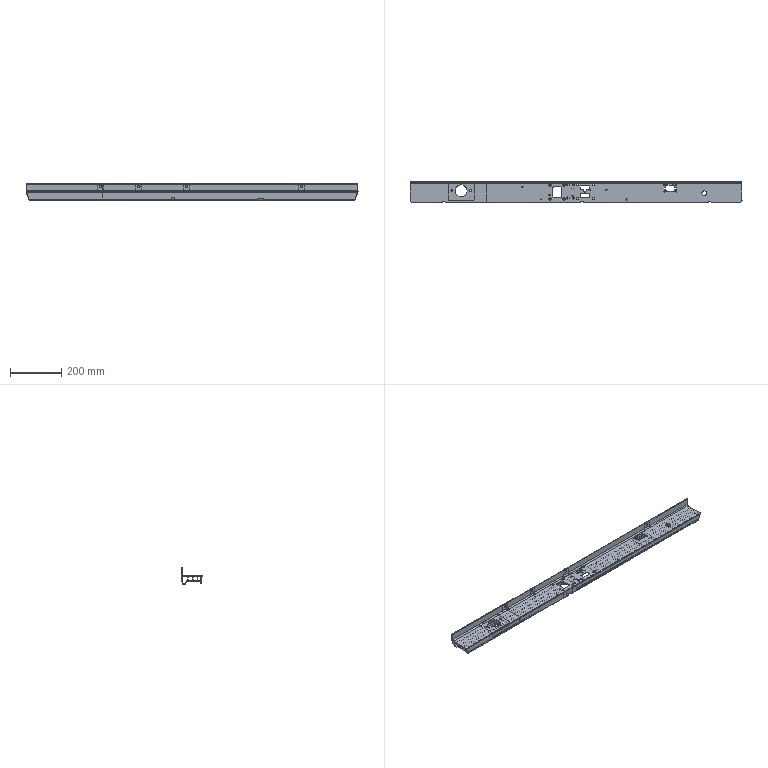NC program | NX | posted with a generic post | part box 1301 x 81.1 x 63 mm
Lines 1 to 1193 of 19815:
N10 G17 G21 G94 G90
(FLOOR_WALL_COPY_COPY , TOOL : D10)
N12 T10 M6
N14 G54
N16 G17 G0 G90 X127.709 Y30.2 B0. C0. S6000 M3
N18 G43 Z30. H10
N20 Z1.5
N22 G94 G1 X107.257 Z0.428 F1000.
N24 Y28.734 Z0.351
N26 X132.857 Z-0.991
N28 X158.457 F2500.
N30 Y30.2
N32 X107.257
N34 Y28.734
N36 X132.857
N38 Y24.234
N40 X162.957
N42 Y34.7
N44 X102.757
N46 Y24.234
N48 X132.857
N50 G2 X133.724 Y23.734 R1.
N52 G1 X134.301 Y22.734
N54 Z0.509
N56 G0 X161.859
N58 G1 Z-0.991 F1000.
N60 X162.957 Y23.368
N62 G3 X163.457 Y24.234 R1.
N64 G1 Y35.2 F2500.
N66 X102.257
N68 Y24.234
N70 G3 X102.757 Y23.368 R1.
N72 G1 X103.856 Y22.734
N74 Z0.509
N76 G0 X127.144 Y30.2
N78 G1 X107.257 Z-0.533 F1000.
N80 Y28.168 Z-0.639
N82 X132.857 Z-1.981
N84 X158.457 F2500.
N86 Y30.2
N88 X107.257
N90 Y28.168
N92 X132.857
N94 Y23.668
N96 X162.957
N98 Y34.7
N100 X102.757
N102 Y23.668
N104 X132.857
N106 G2 X133.724 Y23.168 R1.
N108 G1 X134.301 Y22.168
N110 Z-0.481
N112 G0 X161.859
N114 G1 Z-1.981 F1000.
N116 X162.957 Y22.802
N118 G3 X163.457 Y23.668 R1.
N120 G1 Y35.2 F2500.
N122 X102.257
N124 Y23.668
N126 G3 X102.757 Y22.802 R1.
N128 G1 X103.856 Y22.168
N130 Z-0.481
N132 G0 X126.578 Y30.2
N134 G1 X107.257 Z-1.493 F1000.
N136 Y27.602 Z-1.63
N138 X132.857 Z-2.971
N140 X158.457 F2500.
N142 Y30.2
N144 X107.257
N146 Y27.602
N148 X132.857
N150 Y23.102
N152 X162.957
N154 Y34.7
N156 X102.757
N158 Y23.102
N160 X132.857
N162 G2 X133.724 Y22.602 R1.
N164 G1 X134.301 Y21.602
N166 Z-1.471
N168 G0 X161.859
N170 G1 Z-2.971 F1000.
N172 X162.957 Y22.236
N174 G3 X163.457 Y23.102 R1.
N176 G1 Y35.2 F2500.
N178 X102.257
N180 Y23.102
N182 G3 X102.757 Y22.236 R1.
N184 G1 X103.856 Y21.602
N186 Z-1.471
N188 G0 X126.012 Y30.2
N190 G1 X107.257 Z-2.454 F1000.
N192 Y27.036 Z-2.62
N194 X132.857 Z-3.962
N196 X158.457 F2500.
N198 Y30.2
N200 X107.257
N202 Y27.036
N204 X132.857
N206 Y22.536
N208 X162.957
N210 Y34.7
N212 X102.757
N214 Y22.536
N216 X132.857
N218 G2 X133.724 Y22.036 R1.
N220 G1 X134.301 Y21.036
N222 Z-2.462
N224 G0 X161.859
N226 G1 Z-3.962 F1000.
N228 X162.957 Y21.67
N230 G3 X163.457 Y22.536 R1.
N232 G1 Y35.2 F2500.
N234 X102.257
N236 Y22.536
N238 G3 X102.757 Y21.67 R1.
N240 G1 X103.856 Y21.036
N242 Z-2.462
N244 G0 X140.409 Y26.47
N246 G1 X158.457 Z-3.407 F1000.
N248 Y30.34 Z-3.61
N250 X132.857 Z-4.952
N252 X107.257 F2500.
N254 Y26.47
N256 X158.457
N258 Y30.34
N260 X132.857
N262 Y34.84
N264 X102.757
N266 Y21.97
N268 X162.957
N270 Y34.84
N272 X132.857
N274 Z-3.452
N276 G0 X104.257 Y33.34
N278 G1 Z-4.952 F1000.
N280 X102.324 Y35.09
N282 G3 X102.257 Y34.84 R0.5
N284 G1 Y21.97 F2500.
N286 G3 X102.757 Y21.104 R1.
N288 G1 X103.856 Y20.47
N290 Z-3.452
N292 G0 X161.859
N294 G1 Z-4.952 F1000.
N296 X162.957 Y21.104
N298 G3 X163.457 Y21.97 R1.
N300 G1 Y34.84 F2500.
N302 G3 X163.391 Y35.09 R0.5
N304 G1 X161.457 Y33.34
N306 Z-3.452
N308 G0 X140.409 Y25.904
N310 G1 X158.457 Z-4.398 F1000.
N312 Y29.774 Z-4.601
N314 X132.857 Z-5.942
N316 X107.257 F2500.
N318 Y25.904
N320 X158.457
N322 Y29.774
N324 X132.857
N326 Y34.274
N328 X102.757
N330 Y21.404
N332 X162.957
N334 Y34.274
N336 X132.857
N338 G2 X132.424 Y34.524 R0.5
N340 G1 Z-4.442
N342 G0 X104.257 Y32.774
N344 G1 Z-5.942 F1000.
N346 X102.757 Y35.14
N348 G3 X102.257 Y34.274 R1.
N350 G1 Y21.404 F2500.
N352 G3 X102.757 Y20.538 R1.
N354 G1 X103.856 Y19.904
N356 Z-4.442
N358 G0 X161.859
N360 G1 Z-5.942 F1000.
N362 X162.957 Y20.538
N364 G3 X163.457 Y21.404 R1.
N366 G1 Y34.274 F2500.
N368 G3 X162.957 Y35.14 R1.
N370 G1 X161.457 Y32.774
N372 Z-4.442
N374 G0 X140.409 Y25.339
N376 G1 X158.457 Z-5.388 F1000.
N378 Y29.208 Z-5.591
N380 X132.857 Z-6.932
N382 X107.257 F2500.
N384 Y25.339
N386 X158.457
N388 Y29.208
N390 X132.857
N392 Y33.708
N394 X102.757
N396 Y20.839
N398 X162.957
N400 Y33.708
N402 X132.857
N404 G2 X131.991 Y34.208 R1.
N406 G1 Z-5.432
N408 G0 X104.257 Y32.208
N410 G1 Z-6.932 F1000.
N412 X102.757 Y34.574
N414 G3 X102.257 Y33.708 R1.
N416 G1 Y20.839 F2500.
N418 G3 X102.757 Y19.973 R1.
N420 G1 X103.856 Y19.339
N422 Z-5.432
N424 G0 X161.859
N426 G1 Z-6.932 F1000.
N428 X162.957 Y19.973
N430 G3 X163.457 Y20.839 R1.
N432 G1 Y33.708 F2500.
N434 G3 X162.957 Y34.574 R1.
N436 G1 X161.457 Y32.208
N438 Z-5.432
N440 G0 X140.409 Y24.773
N442 G1 X158.457 Z-6.378 F1000.
N444 Y28.642 Z-6.581
N446 X132.857 Z-7.923
N448 X107.257 F2500.
N450 Y24.773
N452 X158.457
N454 Y28.642
N456 X132.857
N458 Y33.142
N460 X102.757
N462 Y20.273
N464 X162.957
N466 Y33.142
N468 X132.857
N470 G2 X131.991 Y33.642 R1.
N472 G1 Z-6.423
N474 G0 X104.257 Y31.642
N476 G1 Z-7.923 F1000.
N478 X102.757 Y34.008
N480 G3 X102.257 Y33.142 R1.
N482 G1 Y20.273 F2500.
N484 G3 X102.757 Y19.407 R1.
N486 G1 X103.856 Y18.773
N488 Z-6.423
N490 G0 X161.859
N492 G1 Z-7.923 F1000.
N494 X162.957 Y19.407
N496 G3 X163.457 Y20.273 R1.
N498 G1 Y33.142 F2500.
N500 G3 X162.957 Y34.008 R1.
N502 G1 X161.457 Y31.642
N504 Z-6.423
N506 G0 X140.409 Y24.207
N508 G1 X158.457 Z-7.369 F1000.
N510 Y28.076 Z-7.571
N512 X132.857 Z-8.913
N514 X107.257 F2500.
N516 Y24.207
N518 X158.457
N520 Y28.076
N522 X132.857
N524 Y32.576
N526 X102.757
N528 Y19.707
N530 X162.957
N532 Y32.576
N534 X132.857
N536 G2 X131.991 Y33.076 R1.
N538 G1 Z-7.413
N540 G0 X104.257 Y31.076
N542 G1 Z-8.913 F1000.
N544 X102.757 Y33.442
N546 G3 X102.257 Y32.576 R1.
N548 G1 Y19.707 F2500.
N550 G3 X102.757 Y18.841 R1.
N552 G1 X103.856 Y18.207
N554 Z-7.413
N556 G0 X161.859
N558 G1 Z-8.913 F1000.
N560 X162.957 Y18.841
N562 G3 X163.457 Y19.707 R1.
N564 G1 Y32.576 F2500.
N566 G3 X162.957 Y33.442 R1.
N568 G1 X161.457 Y31.076
N570 Z-7.413
N572 G0 X141.011 Y23.039
N574 G1 X158.457 Z-8.327 F1000.
N576 Y27.51 Z-8.562
N578 X132.857 Z-9.903
N580 X107.257 F2500.
N582 Y23.039
N584 X158.457
N586 Y27.51
N588 X132.857
N590 Y32.01
N592 X102.757
N594 Y18.539
N596 X162.957
N598 Y32.01
N600 X132.857
N602 G2 X131.991 Y32.51 R1.
N604 G1 X131.414 Y33.51
N606 Z-8.403
N608 G0 X103.856
N610 G1 Z-9.903 F1000.
N612 X102.757 Y32.876
N614 G3 X102.257 Y32.01 R1.
N616 G1 Y18.539 F2500.
N618 G3 X102.757 Y17.673 R1.
N620 G1 X103.856 Y17.039
N622 Z-8.403
N624 G0 X161.859
N626 G1 Z-9.903 F1000.
N628 X162.957 Y17.673
N630 G3 X163.457 Y18.539 R1.
N632 G1 Y32.01 F2500.
N634 G3 X162.957 Y32.876 R1.
N636 G1 X161.859 Y33.51
N638 Z-8.403
N640 G0 X125.584 Y9.4
N642 G1 X148.957 Z-9.628 F1000.
N644 Y17.444 Z-10.05
N646 X132.857 Z-10.894
N648 X116.757 F2500.
N650 Y9.4
N652 X148.957
N654 Y17.444
N656 X132.857
N658 Y24.444
N660 X109.757
N662 Y2.4
N664 X155.957
N666 Y24.444
N668 X132.857
N670 Y31.444
N672 X102.757
N674 Y-4.6
N676 X162.957
N678 Y31.444
N680 X132.857
N682 G2 X131.991 Y31.944 R1.
N684 G1 X131.414 Y32.944
N686 Z-9.394
N688 G0 X103.856
N690 G1 Z-10.894 F1000.
N692 X102.757 Y32.31
N694 G3 X102.257 Y31.444 R1.
N696 G1 Y-5.1 F2500.
N698 X163.457
N700 Y31.444
N702 G3 X162.957 Y32.31 R1.
N704 G1 X161.859 Y32.944
N706 Z-9.394
N708 G0 X125.018 Y9.4
N710 G1 X148.957 Z-10.648 F1000.
N712 Y16.878 Z-11.04
N714 X132.857 Z-11.884
N716 X116.757 F2500.
N718 Y9.4
N720 X148.957
N722 Y16.878
N724 X132.857
N726 Y23.878
N728 X109.757
N730 Y2.4
N732 X155.957
N734 Y23.878
N736 X132.857
N738 Y30.878
N740 X102.757
N742 Y-4.6
N744 X162.957
N746 Y30.878
N748 X132.857
N750 G2 X131.991 Y31.378 R1.
N752 G1 X131.414 Y32.378
N754 Z-10.384
N756 G0 X103.856
N758 G1 Z-11.884 F1000.
N760 X102.757 Y31.745
N762 G3 X102.257 Y30.878 R1.
N764 G1 Y-5.1 F2500.
N766 X163.457
N768 Y30.878
N770 G3 X162.957 Y31.745 R1.
N772 G1 X161.859 Y32.378
N774 Z-10.384
N776 G0 X124.452 Y9.4
N778 G1 X148.957 Z-11.668 F1000.
N780 Y16.313 Z-12.031
N782 X132.857 Z-12.874
N784 X116.757 F2500.
N786 Y9.4
N788 X148.957
N790 Y16.313
N792 X132.857
N794 Y23.313
N796 X109.757
N798 Y2.4
N800 X155.957
N802 Y23.313
N804 X132.857
N806 Y30.313
N808 X102.757
N810 Y-4.6
N812 X162.957
N814 Y30.313
N816 X132.857
N818 G2 X131.991 Y30.813 R1.
N820 G1 X131.414 Y31.813
N822 Z-11.374
N824 G0 X103.856
N826 G1 Z-12.874 F1000.
N828 X102.757 Y31.179
N830 G3 X102.257 Y30.313 R1.
N832 G1 Y-5.1 F2500.
N834 X163.457
N836 Y30.313
N838 G3 X162.957 Y31.179 R1.
N840 G1 X161.859 Y31.813
N842 Z-11.374
N844 G0 X125.482 Y3.647
N846 G1 X107.257 Z-12.329 F1000.
N848 Y-0.047 Z-12.523
N850 X132.857 Z-13.865
N852 X158.457 F2500.
N854 Y3.647
N856 X107.257
N858 Y-0.047
N860 X132.857
N862 Y-4.547
N864 X162.957
N866 Y8.147
N868 X102.757
N870 Y-4.547
N872 X132.857
N874 G2 X133.107 Y-4.614 R0.5
N876 G1 Z-12.365
N878 G0 X161.457 Y-3.047
N880 G1 Z-13.865 F1000.
N882 X163.207 Y-4.98
N884 G3 X163.457 Y-4.547 R0.5
N886 G1 Y8.147 F2500.
N888 G3 X162.957 Y9.013 R1.
N890 G1 X161.859 Y9.647
N892 Z-12.365
N894 G0 X103.856
N896 G1 Z-13.865 F1000.
N898 X102.757 Y9.013
N900 G3 X102.257 Y8.147 R1.
N902 G1 Y-4.547 F2500.
N904 G3 X102.507 Y-4.98 R0.5
N906 G1 X104.257 Y-3.047
N908 Z-12.365
N910 G0 X126.166 Y3.305
N912 G1 X107.257 Z-13.356 F1000.
N914 Y0.295 Z-13.513
N916 X132.857 Z-14.855
N918 X158.457 F2500.
N920 Y3.305
N922 X107.257
N924 Y0.295
N926 X132.857
N928 Y-4.205
N930 X162.957
N932 Y7.805
N934 X102.757
N936 Y-4.205
N938 X132.857
N940 G2 X133.291 Y-4.455 R0.5
N942 G1 Z-13.355
N944 G0 X161.457 Y-2.705
N946 G1 Z-14.855 F1000.
N948 X162.957 Y-5.071
N950 G3 X163.457 Y-4.205 R1.
N952 G1 Y7.805 F2500.
N954 G3 X162.957 Y8.671 R1.
N956 G1 X161.859 Y9.305
N958 Z-13.355
N960 G0 X103.856
N962 G1 Z-14.855 F1000.
N964 X102.757 Y8.671
N966 G3 X102.257 Y7.805 R1.
N968 G1 Y-4.205 F2500.
N970 G3 X102.757 Y-5.071 R1.
N972 G1 X104.257 Y-2.705
N974 Z-13.355
N976 G0 X126.175 Y3.3
N978 G1 X107.257 Z-14.346 F1000.
N980 Y0.3 Z-14.504
N982 X132.857 Z-15.845
N984 X158.457 F2500.
N986 Y3.3
N988 X107.257
N990 Y0.3
N992 X132.857
N994 Y-4.2
N996 X162.957
N998 Y7.8
N1000 X102.757
N1002 Y-4.2
N1004 X132.857
N1006 G2 X133.291 Y-4.45 R0.5
N1008 G1 Z-14.345
N1010 G0 X161.457 Y-2.7
N1012 G1 Z-15.845 F1000.
N1014 X162.957 Y-5.066
N1016 G3 X163.457 Y-4.2 R1.
N1018 G1 Y7.8 F2500.
N1020 G3 X162.957 Y8.666 R1.
N1022 G1 X161.859 Y9.3
N1024 Z-14.345
N1026 G0 X103.856
N1028 G1 Z-15.845 F1000.
N1030 X102.757 Y8.666
N1032 G3 X102.257 Y7.8 R1.
N1034 G1 Y-4.2 F2500.
N1036 G3 X102.757 Y-5.066 R1.
N1038 G1 X104.257 Y-2.7
N1040 Z-14.345
N1042 G0 X126.175 Y3.3
N1044 G1 X107.257 Z-15.337 F1000.
N1046 Y0.3 Z-15.494
N1048 X132.857 Z-16.836
N1050 X158.457 F2500.
N1052 Y3.3
N1054 X107.257
N1056 Y0.3
N1058 X132.857
N1060 Y-4.2
N1062 X162.957
N1064 Y7.8
N1066 X102.757
N1068 Y-4.2
N1070 X132.857
N1072 G2 X133.291 Y-4.45 R0.5
N1074 G1 Z-15.336
N1076 G0 X161.457 Y-2.7
N1078 G1 Z-16.836 F1000.
N1080 X162.957 Y-5.066
N1082 G3 X163.457 Y-4.2 R1.
N1084 G1 Y7.8 F2500.
N1086 G3 X162.957 Y8.666 R1.
N1088 G1 X161.859 Y9.3
N1090 Z-15.336
N1092 G0 X103.856
N1094 G1 Z-16.836 F1000.
N1096 X102.757 Y8.666
N1098 G3 X102.257 Y7.8 R1.
N1100 G1 Y-4.2 F2500.
N1102 G3 X102.757 Y-5.066 R1.
N1104 G1 X104.257 Y-2.7
N1106 Z-15.336
N1108 G0 X126.175 Y3.3
N1110 G1 X107.257 Z-16.327 F1000.
N1112 Y0.3 Z-16.484
N1114 X132.857 Z-17.826
N1116 X158.457 F2500.
N1118 Y3.3
N1120 X107.257
N1122 Y0.3
N1124 X132.857
N1126 Y-4.2
N1128 X162.957
N1130 Y7.8
N1132 X102.757
N1134 Y-4.2
N1136 X132.857
N1138 G2 X133.291 Y-4.45 R0.5
N1140 G1 Z-16.326
N1142 G0 X161.457 Y-2.7
N1144 G1 Z-17.826 F1000.
N1146 X162.957 Y-5.066
N1148 G3 X163.457 Y-4.2 R1.
N1150 G1 Y7.8 F2500.
N1152 G3 X162.957 Y8.666 R1.
N1154 G1 X161.859 Y9.3
N1156 Z-16.326
N1158 G0 X103.856
N1160 G1 Z-17.826 F1000.
N1162 X102.757 Y8.666
N1164 G3 X102.257 Y7.8 R1.
N1166 G1 Y-4.2 F2500.
N1168 G3 X102.757 Y-5.066 R1.
N1170 G1 X104.257 Y-2.7
N1172 Z-16.326
N1174 G0 X126.175 Y3.3
N1176 G1 X107.257 Z-17.317 F1000.
N1178 Y0.3 Z-17.475
N1180 X132.857 Z-18.816
N1182 X158.457 F2500.
N1184 Y3.3
N1186 X107.257
N1188 Y0.3
N1190 X132.857
N1192 Y-4.2
N1194 X162.957
N1196 Y7.8
N1198 X102.757
N1200 Y-4.2
N1202 X132.857
N1204 G2 X133.291 Y-4.45 R0.5
N1206 G1 Z-17.316
N1208 G0 X161.457 Y-2.7
N1210 G1 Z-18.816 F1000.
N1212 X162.957 Y-5.066
N1214 G3 X163.457 Y-4.2 R1.
N1216 G1 Y7.8 F2500.
N1218 G3 X162.957 Y8.666 R1.
N1220 G1 X161.859 Y9.3
N1222 Z-17.316
N1224 G0 X103.856
N1226 G1 Z-18.816 F1000.
N1228 X102.757 Y8.666
N1230 G3 X102.257 Y7.8 R1.
N1232 G1 Y-4.2 F2500.
N1234 G3 X102.757 Y-5.066 R1.
N1236 G1 X104.257 Y-2.7
N1238 Z-17.316
N1240 G0 X126.175 Y3.3
N1242 G1 X107.257 Z-18.308 F1000.
N1244 Y0.3 Z-18.465
N1246 X132.857 Z-19.807
N1248 X158.457 F2500.
N1250 Y3.3
N1252 X107.257
N1254 Y0.3
N1256 X132.857
N1258 Y-4.2
N1260 X162.957
N1262 Y7.8
N1264 X102.757
N1266 Y-4.2
N1268 X132.857
N1270 G2 X133.291 Y-4.45 R0.5
N1272 G1 Z-18.307
N1274 G0 X161.457 Y-2.7
N1276 G1 Z-19.807 F1000.
N1278 X162.957 Y-5.066
N1280 G3 X163.457 Y-4.2 R1.
N1282 G1 Y7.8 F2500.
N1284 G3 X162.957 Y8.666 R1.
N1286 G1 X161.859 Y9.3
N1288 Z-18.307
N1290 G0 X103.856
N1292 G1 Z-19.807 F1000.
N1294 X102.757 Y8.666
N1296 G3 X102.257 Y7.8 R1.
N1298 G1 Y-4.2 F2500.
N1300 G3 X102.757 Y-5.066 R1.
N1302 G1 X104.257 Y-2.7
N1304 Z-18.307
N1306 G0 X126.175 Y3.3
N1308 G1 X107.257 Z-19.298 F1000.
N1310 Y0.3 Z-19.455
N1312 X132.857 Z-20.797
N1314 X158.457 F2500.
N1316 Y3.3
N1318 X107.257
N1320 Y0.3
N1322 X132.857
N1324 Y-4.2
N1326 X162.957
N1328 Y7.8
N1330 X102.757
N1332 Y-4.2
N1334 X132.857
N1336 G2 X133.291 Y-4.45 R0.5
N1338 G1 Z-19.297
N1340 G0 X161.457 Y-2.7
N1342 G1 Z-20.797 F1000.
N1344 X162.957 Y-5.066
N1346 G3 X163.457 Y-4.2 R1.
N1348 G1 Y7.8 F2500.
N1350 G3 X162.957 Y8.666 R1.
N1352 G1 X161.859 Y9.3
N1354 Z-19.297
N1356 G0 X103.856
N1358 G1 Z-20.797 F1000.
N1360 X102.757 Y8.666
N1362 G3 X102.257 Y7.8 R1.
N1364 G1 Y-4.2 F2500.
N1366 G3 X102.757 Y-5.066 R1.
N1368 G1 X104.257 Y-2.7
N1370 Z-19.297
N1372 G0 X126.175 Y3.3
N1374 G1 X107.257 Z-20.288 F1000.
N1376 Y0.3 Z-20.446
N1378 X132.857 Z-21.787
N1380 X158.457 F2500.
N1382 Y3.3
N1384 X107.257
N1386 Y0.3
N1388 X132.857
N1390 Y-4.2
N1392 X162.957
N1394 Y7.8
N1396 X102.757
N1398 Y-4.2
N1400 X132.857
N1402 G2 X133.291 Y-4.45 R0.5
N1404 G1 Z-20.287
N1406 G0 X161.457 Y-2.7
N1408 G1 Z-21.787 F1000.
N1410 X162.957 Y-5.066
N1412 G3 X163.457 Y-4.2 R1.
N1414 G1 Y7.8 F2500.
N1416 G3 X162.957 Y8.666 R1.
N1418 G1 X161.859 Y9.3
N1420 Z-20.287
N1422 G0 X103.856
N1424 G1 Z-21.787 F1000.
N1426 X102.757 Y8.666
N1428 G3 X102.257 Y7.8 R1.
N1430 G1 Y-4.2 F2500.
N1432 G3 X102.757 Y-5.066 R1.
N1434 G1 X104.257 Y-2.7
N1436 Z-20.287
N1438 G0 X126.175 Y3.3
N1440 G1 X107.257 Z-21.279 F1000.
N1442 Y0.3 Z-21.436
N1444 X132.857 Z-22.777
N1446 X158.457 F2500.
N1448 Y3.3
N1450 X107.257
N1452 Y0.3
N1454 X132.857
N1456 Y-4.2
N1458 X162.957
N1460 Y7.8
N1462 X102.757
N1464 Y-4.2
N1466 X132.857
N1468 G2 X133.291 Y-4.45 R0.5
N1470 G1 Z-21.277
N1472 G0 X161.457 Y-2.7
N1474 G1 Z-22.777 F1000.
N1476 X162.957 Y-5.066
N1478 G3 X163.457 Y-4.2 R1.
N1480 G1 Y7.8 F2500.
N1482 G3 X162.957 Y8.666 R1.
N1484 G1 X161.859 Y9.3
N1486 Z-21.277
N1488 G0 X103.856
N1490 G1 Z-22.777 F1000.
N1492 X102.757 Y8.666
N1494 G3 X102.257 Y7.8 R1.
N1496 G1 Y-4.2 F2500.
N1498 G3 X102.757 Y-5.066 R1.
N1500 G1 X104.257 Y-2.7
N1502 Z-21.277
N1504 G0 X126.175 Y3.3
N1506 G1 X107.257 Z-22.269 F1000.
N1508 Y0.3 Z-22.426
N1510 X132.857 Z-23.768
N1512 X158.457 F2500.
N1514 Y3.3
N1516 X107.257
N1518 Y0.3
N1520 X132.857
N1522 Y-4.2
N1524 X162.957
N1526 Y7.8
N1528 X102.757
N1530 Y-4.2
N1532 X132.857
N1534 G2 X133.291 Y-4.45 R0.5
N1536 G1 Z-22.268
N1538 G0 X161.457 Y-2.7
N1540 G1 Z-23.768 F1000.
N1542 X162.957 Y-5.066
N1544 G3 X163.457 Y-4.2 R1.
N1546 G1 Y7.8 F2500.
N1548 G3 X162.957 Y8.666 R1.
N1550 G1 X161.859 Y9.3
N1552 Z-22.268
N1554 G0 X103.856
N1556 G1 Z-23.768 F1000.
N1558 X102.757 Y8.666
N1560 G3 X102.257 Y7.8 R1.
N1562 G1 Y-4.2 F2500.
N1564 G3 X102.757 Y-5.066 R1.
N1566 G1 X104.257 Y-2.7
N1568 Z-22.268
N1570 G0 X126.175 Y3.3
N1572 G1 X107.257 Z-23.259 F1000.
N1574 Y0.3 Z-23.416
N1576 X132.857 Z-24.758
N1578 X158.457 F2500.
N1580 Y3.3
N1582 X107.257
N1584 Y0.3
N1586 X132.857
N1588 Y-4.2
N1590 X162.957
N1592 Y7.8
N1594 X102.757
N1596 Y-4.2
N1598 X132.857
N1600 G2 X133.291 Y-4.45 R0.5
N1602 G1 Z-23.258
N1604 G0 X161.457 Y-2.7
N1606 G1 Z-24.758 F1000.
N1608 X162.957 Y-5.066
N1610 G3 X163.457 Y-4.2 R1.
N1612 G1 Y7.8 F2500.
N1614 G3 X162.957 Y8.666 R1.
N1616 G1 X161.859 Y9.3
N1618 Z-23.258
N1620 G0 X103.856
N1622 G1 Z-24.758 F1000.
N1624 X102.757 Y8.666
N1626 G3 X102.257 Y7.8 R1.
N1628 G1 Y-4.2 F2500.
N1630 G3 X102.757 Y-5.066 R1.
N1632 G1 X104.257 Y-2.7
N1634 Z-23.258
N1636 G0 X126.175 Y3.3
N1638 G1 X107.257 Z-24.25 F1000.
N1640 Y0.3 Z-24.407
N1642 X132.857 Z-25.748
N1644 X158.457 F2500.
N1646 Y3.3
N1648 X107.257
N1650 Y0.3
N1652 X132.857
N1654 Y-4.2
N1656 X162.957
N1658 Y7.8
N1660 X102.757
N1662 Y-4.2
N1664 X132.857
N1666 G2 X133.291 Y-4.45 R0.5
N1668 G1 Z-24.248
N1670 G0 X161.457 Y-2.7
N1672 G1 Z-25.748 F1000.
N1674 X162.957 Y-5.066
N1676 G3 X163.457 Y-4.2 R1.
N1678 G1 Y7.8 F2500.
N1680 G3 X162.957 Y8.666 R1.
N1682 G1 X161.859 Y9.3
N1684 Z-24.248
N1686 G0 X103.856
N1688 G1 Z-25.748 F1000.
N1690 X102.757 Y8.666
N1692 G3 X102.257 Y7.8 R1.
N1694 G1 Y-4.2 F2500.
N1696 G3 X102.757 Y-5.066 R1.
N1698 G1 X104.257 Y-2.7
N1700 Z-24.248
N1702 G0 X126.175 Y3.3
N1704 G1 X107.257 Z-25.24 F1000.
N1706 Y0.3 Z-25.397
N1708 X132.857 Z-26.739
N1710 X158.457 F2500.
N1712 Y3.3
N1714 X107.257
N1716 Y0.3
N1718 X132.857
N1720 Y-4.2
N1722 X162.957
N1724 Y7.8
N1726 X102.757
N1728 Y-4.2
N1730 X132.857
N1732 G2 X133.291 Y-4.45 R0.5
N1734 G1 Z-25.239
N1736 G0 X161.457 Y-2.7
N1738 G1 Z-26.739 F1000.
N1740 X162.957 Y-5.066
N1742 G3 X163.457 Y-4.2 R1.
N1744 G1 Y7.8 F2500.
N1746 G3 X162.957 Y8.666 R1.
N1748 G1 X161.859 Y9.3
N1750 Z-25.239
N1752 G0 X103.856
N1754 G1 Z-26.739 F1000.
N1756 X102.757 Y8.666
N1758 G3 X102.257 Y7.8 R1.
N1760 G1 Y-4.2 F2500.
N1762 G3 X102.757 Y-5.066 R1.
N1764 G1 X104.257 Y-2.7
N1766 Z-25.239
N1768 G0 X126.175 Y3.3
N1770 G1 X107.257 Z-26.23 F1000.
N1772 Y0.3 Z-26.387
N1774 X132.857 Z-27.729
N1776 X158.457 F2500.
N1778 Y3.3
N1780 X107.257
N1782 Y0.3
N1784 X132.857
N1786 Y-4.2
N1788 X162.957
N1790 Y7.8
N1792 X102.757
N1794 Y-4.2
N1796 X132.857
N1798 G2 X133.291 Y-4.45 R0.5
N1800 G1 Z-26.229
N1802 G0 X161.457 Y-2.7
N1804 G1 Z-27.729 F1000.
N1806 X162.957 Y-5.066
N1808 G3 X163.457 Y-4.2 R1.
N1810 G1 Y7.8 F2500.
N1812 G3 X162.957 Y8.666 R1.
N1814 G1 X161.859 Y9.3
N1816 Z-26.229
N1818 G0 X103.856
N1820 G1 Z-27.729 F1000.
N1822 X102.757 Y8.666
N1824 G3 X102.257 Y7.8 R1.
N1826 G1 Y-4.2 F2500.
N1828 G3 X102.757 Y-5.066 R1.
N1830 G1 X104.257 Y-2.7
N1832 Z-26.229
N1834 G0 X126.163 Y3.3
N1836 G1 X107.257 Z-27.22 F1000.
N1838 Y0.288 Z-27.378
N1840 X132.857 Z-28.719
N1842 X158.457 F2500.
N1844 Y3.3
N1846 X107.257
N1848 Y0.288
N1850 X132.857
N1852 Y-4.212
N1854 X162.957
N1856 Y7.8
N1858 X102.757
N1860 Y-4.212
N1862 X132.857
N1864 G2 X133.291 Y-4.462 R0.5
N1866 G1 Z-27.219
N1868 G0 X161.457 Y-2.712
N1870 G1 Z-28.719 F1000.
N1872 X162.957 Y-5.078
N1874 G3 X163.457 Y-4.212 R1.
N1876 G1 Y7.8 F2500.
N1878 G3 X162.957 Y8.666 R1.
N1880 G1 X161.859 Y9.3
N1882 Z-27.219
N1884 G0 X103.856
N1886 G1 Z-28.719 F1000.
N1888 X102.757 Y8.666
N1890 G3 X102.257 Y7.8 R1.
N1892 G1 Y-4.212 F2500.
N1894 G3 X102.757 Y-5.078 R1.
N1896 G1 X104.257 Y-2.712
N1898 Z-27.219
N1900 G0 X125.746 Y3.322
N1902 G1 X107.257 Z-28.188 F1000.
N1904 Y-0.107 Z-28.368
N1906 X132.857 Z-29.71
N1908 X158.457 F2500.
N1910 Y3.322
N1912 X107.257
N1914 Y-0.107
N1916 X132.857
N1918 Y-4.607
N1920 X162.957
N1922 Y7.822
N1924 X102.757
N1926 Y-4.607
N1928 X132.857
N1930 Z-28.21
N1932 G0 X161.457 Y-3.107
N1934 G1 Z-29.71 F1000.
N1936 X163.207 Y-5.04
N1938 G3 X163.457 Y-4.607 R0.5
N1940 G1 Y7.822 F2500.
N1942 G3 X162.957 Y8.688 R1.
N1944 G1 X161.859 Y9.322
N1946 Z-28.21
N1948 G0 X103.856
N1950 G1 Z-29.71 F1000.
N1952 X102.757 Y8.688
N1954 G3 X102.257 Y7.822 R1.
N1956 G1 Y-4.607 F2500.
N1958 G3 X102.507 Y-5.04 R0.5
N1960 G1 X104.257 Y-3.107
N1962 Z-28.21
N1964 G0 Z30.
N1966 X133.333 Y20.953
N1968 Z-11.374
N1970 G1 X155.957 Z-12.56 F1000.
N1972 Y22.747 Z-12.654
N1974 X132.857 Z-13.865
N1976 X109.757 F2500.
N1978 Y20.953
N1980 X155.957
N1982 Y22.747
N1984 X132.857
N1986 Y29.747
N1988 X102.757
N1990 Y13.953
N1992 X162.957
N1994 Y29.747
N1996 X132.857
N1998 G2 X131.991 Y30.247 R1.
N2000 G1 X131.414 Y31.247
N2002 Z-12.365
N2004 G0 X103.856
N2006 G1 Z-13.865 F1000.
N2008 X102.757 Y30.613
N2010 G3 X102.257 Y29.747 R1.
N2012 G1 Y13.953 F2500.
N2014 G3 X102.757 Y13.087 R1.
N2016 G1 X103.856 Y12.453
N2018 Z-12.365
N2020 G0 X161.859
N2022 G1 Z-13.865 F1000.
N2024 X162.957 Y13.087
N2026 G3 X163.457 Y13.953 R1.
N2028 G1 Y29.747 F2500.
N2030 G3 X162.957 Y30.613 R1.
N2032 G1 X161.859 Y31.247
N2034 Z-12.365
N2036 G0 X132.425 Y21.295
N2038 G1 X155.957 Z-13.598 F1000.
N2040 Y22.181 Z-13.644
N2042 X132.857 Z-14.855
N2044 X109.757 F2500.
N2046 Y21.295
N2048 X155.957
N2050 Y22.181
N2052 X132.857
N2054 Y29.181
N2056 X102.757
N2058 Y14.295
N2060 X162.957
N2062 Y29.181
N2064 X132.857
N2066 G2 X131.991 Y29.681 R1.
N2068 G1 X131.414 Y30.681
N2070 Z-13.355
N2072 G0 X103.856
N2074 G1 Z-14.855 F1000.
N2076 X102.757 Y30.047
N2078 G3 X102.257 Y29.181 R1.
N2080 G1 Y14.295 F2500.
N2082 G3 X102.757 Y13.429 R1.
N2084 G1 X103.856 Y12.795
N2086 Z-13.355
N2088 G0 X161.859
N2090 G1 Z-14.855 F1000.
N2092 X162.957 Y13.429
N2094 G3 X163.457 Y14.295 R1.
N2096 G1 Y29.181 F2500.
N2098 G3 X162.957 Y30.047 R1.
N2100 G1 X161.859 Y30.681
N2102 Z-13.355
N2104 G0 X133.861 Y21.615
N2106 G1 X109.757 Z-14.618 F1000.
N2108 Y21.3 Z-14.635
N2110 X132.857 Z-15.845
N2112 X155.957 F2500.
N2114 Y21.615
N2116 X109.757
N2118 Y21.3
N2120 X132.857
N2122 Y14.3
N2124 X162.957
N2126 Y28.615
N2128 X102.757
N2130 Y14.3
N2132 X132.857
N2134 G2 X133.724 Y13.8 R1.
N2136 G1 X134.301 Y12.8
N2138 Z-14.345
N2140 G0 X161.859
N2142 G1 Z-15.845 F1000.
N2144 X162.957 Y13.434
N2146 G3 X163.457 Y14.3 R1.
N2148 G1 Y28.615 F2500.
N2150 G3 X162.957 Y29.481 R1.
N2152 G1 X161.859 Y30.115
N2154 Z-14.345
N2156 G0 X103.856
N2158 G1 Z-15.845 F1000.
N2160 X102.757 Y29.481
N2162 G3 X102.257 Y28.615 R1.
N2164 G1 Y14.3 F2500.
N2166 G3 X102.757 Y13.434 R1.
N2168 G1 X103.856 Y12.8
N2170 Z-14.345
N2172 G0 X141.288 Y18.8
N2174 G1 X158.457 Z-15.245 F1000.
N2176 Y23.549 Z-15.494
N2178 X132.857 Z-16.836
N2180 X107.257 F2500.
N2182 Y18.8
N2184 X158.457
N2186 Y23.549
N2188 X132.857
N2190 Y28.049
N2192 X102.757
N2194 Y14.3
N2196 X162.957
N2198 Y28.049
N2200 X132.857
N2202 G2 X131.991 Y28.549 R1.
N2204 G1 X131.414 Y29.549
N2206 Z-15.336
N2208 G0 X103.856
N2210 G1 Z-16.836 F1000.
N2212 X102.757 Y28.915
N2214 G3 X102.257 Y28.049 R1.
N2216 G1 Y14.3 F2500.
N2218 G3 X102.757 Y13.434 R1.
N2220 G1 X103.856 Y12.8
N2222 Z-15.336
N2224 G0 X161.859
N2226 G1 Z-16.836 F1000.
N2228 X162.957 Y13.434
N2230 G3 X163.457 Y14.3 R1.
N2232 G1 Y28.049 F2500.
N2234 G3 X162.957 Y28.915 R1.
N2236 G1 X161.859 Y29.549
N2238 Z-15.336
N2240 G0 X140.723 Y18.8
N2242 G1 X158.457 Z-16.265 F1000.
N2244 Y22.983 Z-16.484
N2246 X132.857 Z-17.826
N2248 X107.257 F2500.
N2250 Y18.8
N2252 X158.457
N2254 Y22.983
N2256 X132.857
N2258 Y27.483
N2260 X102.757
N2262 Y14.3
N2264 X162.957
N2266 Y27.483
N2268 X132.857
N2270 G2 X131.991 Y27.983 R1.
N2272 G1 X131.414 Y28.983
N2274 Z-16.326
N2276 G0 X103.856
N2278 G1 Z-17.826 F1000.
N2280 X102.757 Y28.349
N2282 G3 X102.257 Y27.483 R1.
N2284 G1 Y14.3 F2500.
N2286 G3 X102.757 Y13.434 R1.
N2288 G1 X103.856 Y12.8
N2290 Z-16.326
N2292 G0 X161.859
N2294 G1 Z-17.826 F1000.
N2296 X162.957 Y13.434
N2298 G3 X163.457 Y14.3 R1.
N2300 G1 Y27.483 F2500.
N2302 G3 X162.957 Y28.349 R1.
N2304 G1 X161.859 Y28.983
N2306 Z-16.326
N2308 G0 X140.157 Y18.8
N2310 G1 X158.457 Z-17.285 F1000.
N2312 Y22.417 Z-17.475
N2314 X132.857 Z-18.816
N2316 X107.257 F2500.
N2318 Y18.8
N2320 X158.457
N2322 Y22.417
N2324 X132.857
N2326 Y26.917
N2328 X102.757
N2330 Y14.3
N2332 X162.957
N2334 Y26.917
N2336 X132.857
N2338 G2 X131.991 Y27.417 R1.
N2340 G1 X131.414 Y28.417
N2342 Z-17.316
N2344 G0 X103.856
N2346 G1 Z-18.816 F1000.
N2348 X102.757 Y27.783
N2350 G3 X102.257 Y26.917 R1.
N2352 G1 Y14.3 F2500.
N2354 G3 X102.757 Y13.434 R1.
N2356 G1 X103.856 Y12.8
N2358 Z-17.316
N2360 G0 X161.859
N2362 G1 Z-18.816 F1000.
N2364 X162.957 Y13.434
N2366 G3 X163.457 Y14.3 R1.
N2368 G1 Y26.917 F2500.
N2370 G3 X162.957 Y27.783 R1.
N2372 G1 X161.859 Y28.417
N2374 Z-17.316
N2376 G0 X139.638 Y18.8
N2378 G1 X158.457 Z-18.303 F1000.
N2380 Y21.899 Z-18.465
N2382 X132.857 Z-19.807
N2384 X107.257 F2500.